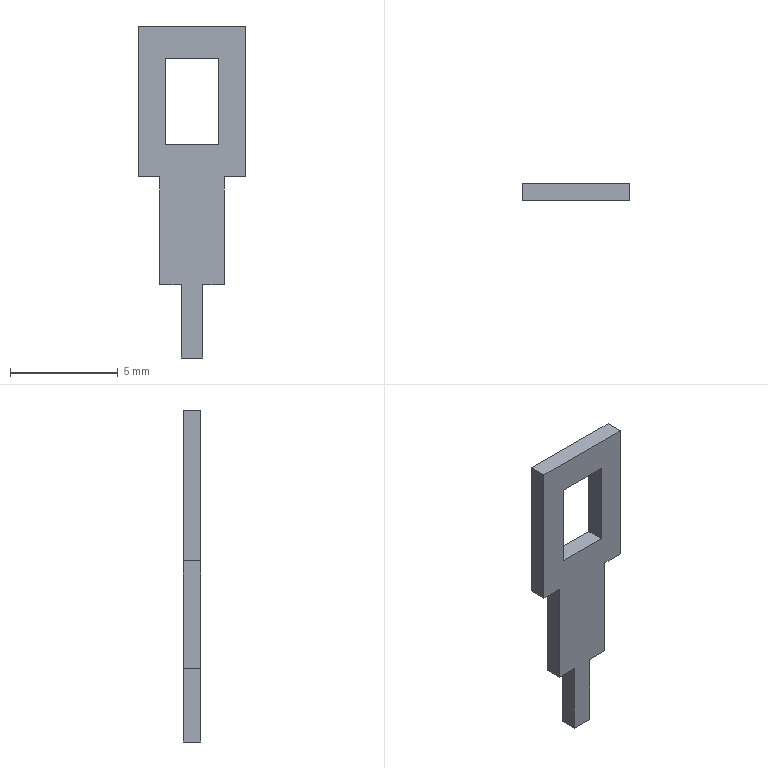Part | STEP file | LRS-150-12_X2_5F00517375-151318 | 1 solid | 18 faces | box 5 x 0.8 x 15.4 mm | volume 34.72 mm3 | plane 18
STEP:
#1=CARTESIAN_POINT('',(0.,0.,0.));
#2=DIRECTION('',(0.,0.,1.));
#3=DIRECTION('',(1.,0.,0.));
#4=AXIS2_PLACEMENT_3D('',#1,#2,#3);
#5=CARTESIAN_POINT('',(-241.667,262.225,6.5));
#6=VERTEX_POINT('',#5);
#7=CARTESIAN_POINT('',(-241.667,263.025,6.5));
#8=VERTEX_POINT('',#7);
#9=CARTESIAN_POINT('',(-241.667,262.225,6.5));
#10=DIRECTION('',(0.,1.,0.));
#11=VECTOR('',#10,1.);
#12=LINE('',#9,#11);
#13=CARTESIAN_POINT('',(-241.667,262.225,6.5));
#14=DIRECTION('',(0.,0.,1.));
#15=DIRECTION('',(1.,0.,0.));
#16=AXIS2_PLACEMENT_3D('',#13,#14,#15);
#17=PLANE('',#16);
#18=CARTESIAN_POINT('',(0.,0.));
#19=DIRECTION('',(0.,1.));
#20=VECTOR('',#19,1.);
#21=LINE('',#18,#20);
#22=(GEOMETRIC_REPRESENTATION_CONTEXT(2)PARAMETRIC_REPRESENTATION_CONTEXT()REPRESENTATION_CONTEXT('',''));
#23=DEFINITIONAL_REPRESENTATION('',(#21),#22);
#24=PCURVE('',#17,#23);
#25=CARTESIAN_POINT('',(-241.667,262.225,10.5));
#26=DIRECTION('',(-1.,0.,0.));
#27=DIRECTION('',(0.,0.,1.));
#28=AXIS2_PLACEMENT_3D('',#25,#26,#27);
#29=PLANE('',#28);
#30=CARTESIAN_POINT('',(-4.,0.));
#31=DIRECTION('',(0.,1.));
#32=VECTOR('',#31,1.);
#33=LINE('',#30,#32);
#34=(GEOMETRIC_REPRESENTATION_CONTEXT(2)PARAMETRIC_REPRESENTATION_CONTEXT()REPRESENTATION_CONTEXT('',''));
#35=DEFINITIONAL_REPRESENTATION('',(#33),#34);
#36=PCURVE('',#29,#35);
#37=SURFACE_CURVE('',#12,(#24,#36),.PCURVE_S1.);
#38=EDGE_CURVE('',#6,#8,#37,.T.);
#39=ORIENTED_EDGE('',*,*,#38,.F.);
#40=CARTESIAN_POINT('',(-244.167,262.225,6.5));
#41=VERTEX_POINT('',#40);
#42=CARTESIAN_POINT('',(-244.167,262.225,6.5));
#43=DIRECTION('',(1.,0.,0.));
#44=VECTOR('',#43,1.);
#45=LINE('',#42,#44);
#46=CARTESIAN_POINT('',(-2.5,0.));
#47=DIRECTION('',(1.,0.));
#48=VECTOR('',#47,1.);
#49=LINE('',#46,#48);
#50=(GEOMETRIC_REPRESENTATION_CONTEXT(2)PARAMETRIC_REPRESENTATION_CONTEXT()REPRESENTATION_CONTEXT('',''));
#51=DEFINITIONAL_REPRESENTATION('',(#49),#50);
#52=PCURVE('',#17,#51);
#53=CARTESIAN_POINT('',(-250.446,262.225,19.929));
#54=DIRECTION('',(0.,1.,0.));
#55=DIRECTION('',(1.,0.,0.));
#56=AXIS2_PLACEMENT_3D('',#53,#54,#55);
#57=PLANE('',#56);
#58=CARTESIAN_POINT('',(6.28,13.429));
#59=DIRECTION('',(1.,0.));
#60=VECTOR('',#59,1.);
#61=LINE('',#58,#60);
#62=(GEOMETRIC_REPRESENTATION_CONTEXT(2)PARAMETRIC_REPRESENTATION_CONTEXT()REPRESENTATION_CONTEXT('',''));
#63=DEFINITIONAL_REPRESENTATION('',(#61),#62);
#64=PCURVE('',#57,#63);
#65=SURFACE_CURVE('',#45,(#52,#64),.PCURVE_S1.);
#66=EDGE_CURVE('',#41,#6,#65,.T.);
#67=ORIENTED_EDGE('',*,*,#66,.F.);
#68=CARTESIAN_POINT('',(-244.167,263.025,6.5));
#69=VERTEX_POINT('',#68);
#70=CARTESIAN_POINT('',(-244.167,262.225,6.5));
#71=DIRECTION('',(0.,1.,0.));
#72=VECTOR('',#71,1.);
#73=LINE('',#70,#72);
#74=CARTESIAN_POINT('',(-2.5,0.));
#75=DIRECTION('',(0.,1.));
#76=VECTOR('',#75,1.);
#77=LINE('',#74,#76);
#78=(GEOMETRIC_REPRESENTATION_CONTEXT(2)PARAMETRIC_REPRESENTATION_CONTEXT()REPRESENTATION_CONTEXT('',''));
#79=DEFINITIONAL_REPRESENTATION('',(#77),#78);
#80=PCURVE('',#17,#79);
#81=CARTESIAN_POINT('',(-244.167,262.225,6.5));
#82=DIRECTION('',(1.,0.,0.));
#83=DIRECTION('',(0.,0.,-1.));
#84=AXIS2_PLACEMENT_3D('',#81,#82,#83);
#85=PLANE('',#84);
#86=CARTESIAN_POINT('',(0.,0.));
#87=DIRECTION('',(0.,1.));
#88=VECTOR('',#87,1.);
#89=LINE('',#86,#88);
#90=(GEOMETRIC_REPRESENTATION_CONTEXT(2)PARAMETRIC_REPRESENTATION_CONTEXT()REPRESENTATION_CONTEXT('',''));
#91=DEFINITIONAL_REPRESENTATION('',(#89),#90);
#92=PCURVE('',#85,#91);
#93=SURFACE_CURVE('',#73,(#80,#92),.PCURVE_S1.);
#94=EDGE_CURVE('',#41,#69,#93,.T.);
#95=ORIENTED_EDGE('',*,*,#94,.T.);
#96=CARTESIAN_POINT('',(-244.167,263.025,6.5));
#97=DIRECTION('',(1.,0.,0.));
#98=VECTOR('',#97,1.);
#99=LINE('',#96,#98);
#100=CARTESIAN_POINT('',(-2.5,0.8));
#101=DIRECTION('',(1.,0.));
#102=VECTOR('',#101,1.);
#103=LINE('',#100,#102);
#104=(GEOMETRIC_REPRESENTATION_CONTEXT(2)PARAMETRIC_REPRESENTATION_CONTEXT()REPRESENTATION_CONTEXT('',''));
#105=DEFINITIONAL_REPRESENTATION('',(#103),#104);
#106=PCURVE('',#17,#105);
#107=CARTESIAN_POINT('',(-250.446,263.025,19.929));
#108=DIRECTION('',(0.,1.,0.));
#109=DIRECTION('',(1.,0.,0.));
#110=AXIS2_PLACEMENT_3D('',#107,#108,#109);
#111=PLANE('',#110);
#112=CARTESIAN_POINT('',(6.28,13.429));
#113=DIRECTION('',(1.,0.));
#114=VECTOR('',#113,1.);
#115=LINE('',#112,#114);
#116=(GEOMETRIC_REPRESENTATION_CONTEXT(2)PARAMETRIC_REPRESENTATION_CONTEXT()REPRESENTATION_CONTEXT('',''));
#117=DEFINITIONAL_REPRESENTATION('',(#115),#116);
#118=PCURVE('',#111,#117);
#119=SURFACE_CURVE('',#99,(#106,#118),.PCURVE_S1.);
#120=EDGE_CURVE('',#69,#8,#119,.T.);
#121=ORIENTED_EDGE('',*,*,#120,.T.);
#122=EDGE_LOOP('',(#39,#67,#95,#121));
#123=FACE_BOUND('',#122,.F.);
#124=ADVANCED_FACE('',(#123),#17,.T.);
#125=CARTESIAN_POINT('',(-241.667,262.225,10.5));
#126=VERTEX_POINT('',#125);
#127=CARTESIAN_POINT('',(-241.667,263.025,10.5));
#128=VERTEX_POINT('',#127);
#129=CARTESIAN_POINT('',(-241.667,262.225,10.5));
#130=DIRECTION('',(0.,1.,0.));
#131=VECTOR('',#130,1.);
#132=LINE('',#129,#131);
#133=CARTESIAN_POINT('',(0.,0.));
#134=DIRECTION('',(0.,1.));
#135=VECTOR('',#134,1.);
#136=LINE('',#133,#135);
#137=(GEOMETRIC_REPRESENTATION_CONTEXT(2)PARAMETRIC_REPRESENTATION_CONTEXT()REPRESENTATION_CONTEXT('',''));
#138=DEFINITIONAL_REPRESENTATION('',(#136),#137);
#139=PCURVE('',#29,#138);
#140=CARTESIAN_POINT('',(-244.167,262.225,10.5));
#141=DIRECTION('',(0.,0.,-1.));
#142=DIRECTION('',(-1.,0.,0.));
#143=AXIS2_PLACEMENT_3D('',#140,#141,#142);
#144=PLANE('',#143);
#145=CARTESIAN_POINT('',(-2.5,0.));
#146=DIRECTION('',(0.,1.));
#147=VECTOR('',#146,1.);
#148=LINE('',#145,#147);
#149=(GEOMETRIC_REPRESENTATION_CONTEXT(2)PARAMETRIC_REPRESENTATION_CONTEXT()REPRESENTATION_CONTEXT('',''));
#150=DEFINITIONAL_REPRESENTATION('',(#148),#149);
#151=PCURVE('',#144,#150);
#152=SURFACE_CURVE('',#132,(#139,#151),.PCURVE_S1.);
#153=EDGE_CURVE('',#126,#128,#152,.T.);
#154=ORIENTED_EDGE('',*,*,#153,.F.);
#155=CARTESIAN_POINT('',(-241.667,262.225,6.5));
#156=DIRECTION('',(0.,0.,1.));
#157=VECTOR('',#156,1.);
#158=LINE('',#155,#157);
#159=CARTESIAN_POINT('',(-4.,0.));
#160=DIRECTION('',(1.,0.));
#161=VECTOR('',#160,1.);
#162=LINE('',#159,#161);
#163=(GEOMETRIC_REPRESENTATION_CONTEXT(2)PARAMETRIC_REPRESENTATION_CONTEXT()REPRESENTATION_CONTEXT('',''));
#164=DEFINITIONAL_REPRESENTATION('',(#162),#163);
#165=PCURVE('',#29,#164);
#166=CARTESIAN_POINT('',(8.78,13.429));
#167=DIRECTION('',(0.,-1.));
#168=VECTOR('',#167,1.);
#169=LINE('',#166,#168);
#170=(GEOMETRIC_REPRESENTATION_CONTEXT(2)PARAMETRIC_REPRESENTATION_CONTEXT()REPRESENTATION_CONTEXT('',''));
#171=DEFINITIONAL_REPRESENTATION('',(#169),#170);
#172=PCURVE('',#57,#171);
#173=SURFACE_CURVE('',#158,(#165,#172),.PCURVE_S1.);
#174=EDGE_CURVE('',#6,#126,#173,.T.);
#175=ORIENTED_EDGE('',*,*,#174,.F.);
#176=ORIENTED_EDGE('',*,*,#38,.T.);
#177=CARTESIAN_POINT('',(-241.667,263.025,6.5));
#178=DIRECTION('',(0.,0.,1.));
#179=VECTOR('',#178,1.);
#180=LINE('',#177,#179);
#181=CARTESIAN_POINT('',(-4.,0.8));
#182=DIRECTION('',(1.,0.));
#183=VECTOR('',#182,1.);
#184=LINE('',#181,#183);
#185=(GEOMETRIC_REPRESENTATION_CONTEXT(2)PARAMETRIC_REPRESENTATION_CONTEXT()REPRESENTATION_CONTEXT('',''));
#186=DEFINITIONAL_REPRESENTATION('',(#184),#185);
#187=PCURVE('',#29,#186);
#188=CARTESIAN_POINT('',(8.78,13.429));
#189=DIRECTION('',(0.,-1.));
#190=VECTOR('',#189,1.);
#191=LINE('',#188,#190);
#192=(GEOMETRIC_REPRESENTATION_CONTEXT(2)PARAMETRIC_REPRESENTATION_CONTEXT()REPRESENTATION_CONTEXT('',''));
#193=DEFINITIONAL_REPRESENTATION('',(#191),#192);
#194=PCURVE('',#111,#193);
#195=SURFACE_CURVE('',#180,(#187,#194),.PCURVE_S1.);
#196=EDGE_CURVE('',#8,#128,#195,.T.);
#197=ORIENTED_EDGE('',*,*,#196,.T.);
#198=EDGE_LOOP('',(#154,#175,#176,#197));
#199=FACE_BOUND('',#198,.F.);
#200=ADVANCED_FACE('',(#199),#29,.T.);
#201=CARTESIAN_POINT('',(-244.167,262.225,10.5));
#202=VERTEX_POINT('',#201);
#203=CARTESIAN_POINT('',(-244.167,263.025,10.5));
#204=VERTEX_POINT('',#203);
#205=CARTESIAN_POINT('',(-244.167,262.225,10.5));
#206=DIRECTION('',(0.,1.,0.));
#207=VECTOR('',#206,1.);
#208=LINE('',#205,#207);
#209=CARTESIAN_POINT('',(0.,0.));
#210=DIRECTION('',(0.,1.));
#211=VECTOR('',#210,1.);
#212=LINE('',#209,#211);
#213=(GEOMETRIC_REPRESENTATION_CONTEXT(2)PARAMETRIC_REPRESENTATION_CONTEXT()REPRESENTATION_CONTEXT('',''));
#214=DEFINITIONAL_REPRESENTATION('',(#212),#213);
#215=PCURVE('',#144,#214);
#216=CARTESIAN_POINT('',(-4.,0.));
#217=DIRECTION('',(0.,1.));
#218=VECTOR('',#217,1.);
#219=LINE('',#216,#218);
#220=(GEOMETRIC_REPRESENTATION_CONTEXT(2)PARAMETRIC_REPRESENTATION_CONTEXT()REPRESENTATION_CONTEXT('',''));
#221=DEFINITIONAL_REPRESENTATION('',(#219),#220);
#222=PCURVE('',#85,#221);
#223=SURFACE_CURVE('',#208,(#215,#222),.PCURVE_S1.);
#224=EDGE_CURVE('',#202,#204,#223,.T.);
#225=ORIENTED_EDGE('',*,*,#224,.F.);
#226=CARTESIAN_POINT('',(-241.667,262.225,10.5));
#227=DIRECTION('',(-1.,0.,0.));
#228=VECTOR('',#227,1.);
#229=LINE('',#226,#228);
#230=CARTESIAN_POINT('',(-2.5,0.));
#231=DIRECTION('',(1.,0.));
#232=VECTOR('',#231,1.);
#233=LINE('',#230,#232);
#234=(GEOMETRIC_REPRESENTATION_CONTEXT(2)PARAMETRIC_REPRESENTATION_CONTEXT()REPRESENTATION_CONTEXT('',''));
#235=DEFINITIONAL_REPRESENTATION('',(#233),#234);
#236=PCURVE('',#144,#235);
#237=CARTESIAN_POINT('',(8.78,9.429));
#238=DIRECTION('',(-1.,0.));
#239=VECTOR('',#238,1.);
#240=LINE('',#237,#239);
#241=(GEOMETRIC_REPRESENTATION_CONTEXT(2)PARAMETRIC_REPRESENTATION_CONTEXT()REPRESENTATION_CONTEXT('',''));
#242=DEFINITIONAL_REPRESENTATION('',(#240),#241);
#243=PCURVE('',#57,#242);
#244=SURFACE_CURVE('',#229,(#236,#243),.PCURVE_S1.);
#245=EDGE_CURVE('',#126,#202,#244,.T.);
#246=ORIENTED_EDGE('',*,*,#245,.F.);
#247=ORIENTED_EDGE('',*,*,#153,.T.);
#248=CARTESIAN_POINT('',(-241.667,263.025,10.5));
#249=DIRECTION('',(-1.,0.,0.));
#250=VECTOR('',#249,1.);
#251=LINE('',#248,#250);
#252=CARTESIAN_POINT('',(-2.5,0.8));
#253=DIRECTION('',(1.,0.));
#254=VECTOR('',#253,1.);
#255=LINE('',#252,#254);
#256=(GEOMETRIC_REPRESENTATION_CONTEXT(2)PARAMETRIC_REPRESENTATION_CONTEXT()REPRESENTATION_CONTEXT('',''));
#257=DEFINITIONAL_REPRESENTATION('',(#255),#256);
#258=PCURVE('',#144,#257);
#259=CARTESIAN_POINT('',(8.78,9.429));
#260=DIRECTION('',(-1.,0.));
#261=VECTOR('',#260,1.);
#262=LINE('',#259,#261);
#263=(GEOMETRIC_REPRESENTATION_CONTEXT(2)PARAMETRIC_REPRESENTATION_CONTEXT()REPRESENTATION_CONTEXT('',''));
#264=DEFINITIONAL_REPRESENTATION('',(#262),#263);
#265=PCURVE('',#111,#264);
#266=SURFACE_CURVE('',#251,(#258,#265),.PCURVE_S1.);
#267=EDGE_CURVE('',#128,#204,#266,.T.);
#268=ORIENTED_EDGE('',*,*,#267,.T.);
#269=EDGE_LOOP('',(#225,#246,#247,#268));
#270=FACE_BOUND('',#269,.F.);
#271=ADVANCED_FACE('',(#270),#144,.T.);
#272=ORIENTED_EDGE('',*,*,#94,.F.);
#273=CARTESIAN_POINT('',(-244.167,262.225,10.5));
#274=DIRECTION('',(0.,0.,-1.));
#275=VECTOR('',#274,1.);
#276=LINE('',#273,#275);
#277=CARTESIAN_POINT('',(-4.,0.));
#278=DIRECTION('',(1.,0.));
#279=VECTOR('',#278,1.);
#280=LINE('',#277,#279);
#281=(GEOMETRIC_REPRESENTATION_CONTEXT(2)PARAMETRIC_REPRESENTATION_CONTEXT()REPRESENTATION_CONTEXT('',''));
#282=DEFINITIONAL_REPRESENTATION('',(#280),#281);
#283=PCURVE('',#85,#282);
#284=CARTESIAN_POINT('',(6.28,9.429));
#285=DIRECTION('',(0.,1.));
#286=VECTOR('',#285,1.);
#287=LINE('',#284,#286);
#288=(GEOMETRIC_REPRESENTATION_CONTEXT(2)PARAMETRIC_REPRESENTATION_CONTEXT()REPRESENTATION_CONTEXT('',''));
#289=DEFINITIONAL_REPRESENTATION('',(#287),#288);
#290=PCURVE('',#57,#289);
#291=SURFACE_CURVE('',#276,(#283,#290),.PCURVE_S1.);
#292=EDGE_CURVE('',#202,#41,#291,.T.);
#293=ORIENTED_EDGE('',*,*,#292,.F.);
#294=ORIENTED_EDGE('',*,*,#224,.T.);
#295=CARTESIAN_POINT('',(-244.167,263.025,10.5));
#296=DIRECTION('',(0.,0.,-1.));
#297=VECTOR('',#296,1.);
#298=LINE('',#295,#297);
#299=CARTESIAN_POINT('',(-4.,0.8));
#300=DIRECTION('',(1.,0.));
#301=VECTOR('',#300,1.);
#302=LINE('',#299,#301);
#303=(GEOMETRIC_REPRESENTATION_CONTEXT(2)PARAMETRIC_REPRESENTATION_CONTEXT()REPRESENTATION_CONTEXT('',''));
#304=DEFINITIONAL_REPRESENTATION('',(#302),#303);
#305=PCURVE('',#85,#304);
#306=CARTESIAN_POINT('',(6.28,9.429));
#307=DIRECTION('',(0.,1.));
#308=VECTOR('',#307,1.);
#309=LINE('',#306,#308);
#310=(GEOMETRIC_REPRESENTATION_CONTEXT(2)PARAMETRIC_REPRESENTATION_CONTEXT()REPRESENTATION_CONTEXT('',''));
#311=DEFINITIONAL_REPRESENTATION('',(#309),#310);
#312=PCURVE('',#111,#311);
#313=SURFACE_CURVE('',#298,(#305,#312),.PCURVE_S1.);
#314=EDGE_CURVE('',#204,#69,#313,.T.);
#315=ORIENTED_EDGE('',*,*,#314,.T.);
#316=EDGE_LOOP('',(#272,#293,#294,#315));
#317=FACE_BOUND('',#316,.F.);
#318=ADVANCED_FACE('',(#317),#85,.T.);
#319=CARTESIAN_POINT('',(-242.417,262.225,0.));
#320=VERTEX_POINT('',#319);
#321=CARTESIAN_POINT('',(-241.417,262.225,0.));
#322=VERTEX_POINT('',#321);
#323=CARTESIAN_POINT('',(-242.417,262.225,0.));
#324=DIRECTION('',(1.,0.,0.));
#325=VECTOR('',#324,1.);
#326=LINE('',#323,#325);
#327=CARTESIAN_POINT('',(8.03,19.929));
#328=DIRECTION('',(1.,0.));
#329=VECTOR('',#328,1.);
#330=LINE('',#327,#329);
#331=(GEOMETRIC_REPRESENTATION_CONTEXT(2)PARAMETRIC_REPRESENTATION_CONTEXT()REPRESENTATION_CONTEXT('',''));
#332=DEFINITIONAL_REPRESENTATION('',(#330),#331);
#333=PCURVE('',#57,#332);
#334=CARTESIAN_POINT('',(-242.417,262.225,0.));
#335=DIRECTION('',(0.,0.,-1.));
#336=DIRECTION('',(-1.,0.,0.));
#337=AXIS2_PLACEMENT_3D('',#334,#335,#336);
#338=PLANE('',#337);
#339=CARTESIAN_POINT('',(0.,0.));
#340=DIRECTION('',(-1.,0.));
#341=VECTOR('',#340,1.);
#342=LINE('',#339,#341);
#343=(GEOMETRIC_REPRESENTATION_CONTEXT(2)PARAMETRIC_REPRESENTATION_CONTEXT()REPRESENTATION_CONTEXT('',''));
#344=DEFINITIONAL_REPRESENTATION('',(#342),#343);
#345=PCURVE('',#338,#344);
#346=SURFACE_CURVE('',#326,(#333,#345),.PCURVE_S1.);
#347=EDGE_CURVE('',#320,#322,#346,.T.);
#348=ORIENTED_EDGE('',*,*,#347,.F.);
#349=CARTESIAN_POINT('',(-242.417,262.225,-3.4));
#350=VERTEX_POINT('',#349);
#351=CARTESIAN_POINT('',(-242.417,262.225,-3.4));
#352=DIRECTION('',(0.,0.,1.));
#353=VECTOR('',#352,1.);
#354=LINE('',#351,#353);
#355=CARTESIAN_POINT('',(8.03,23.329));
#356=DIRECTION('',(0.,-1.));
#357=VECTOR('',#356,1.);
#358=LINE('',#355,#357);
#359=(GEOMETRIC_REPRESENTATION_CONTEXT(2)PARAMETRIC_REPRESENTATION_CONTEXT()REPRESENTATION_CONTEXT('',''));
#360=DEFINITIONAL_REPRESENTATION('',(#358),#359);
#361=PCURVE('',#57,#360);
#362=CARTESIAN_POINT('',(-242.417,262.225,-3.4));
#363=DIRECTION('',(1.,0.,0.));
#364=DIRECTION('',(0.,0.,-1.));
#365=AXIS2_PLACEMENT_3D('',#362,#363,#364);
#366=PLANE('',#365);
#367=CARTESIAN_POINT('',(0.,0.));
#368=DIRECTION('',(-1.,0.));
#369=VECTOR('',#368,1.);
#370=LINE('',#367,#369);
#371=(GEOMETRIC_REPRESENTATION_CONTEXT(2)PARAMETRIC_REPRESENTATION_CONTEXT()REPRESENTATION_CONTEXT('',''));
#372=DEFINITIONAL_REPRESENTATION('',(#370),#371);
#373=PCURVE('',#366,#372);
#374=SURFACE_CURVE('',#354,(#361,#373),.PCURVE_S1.);
#375=EDGE_CURVE('',#350,#320,#374,.T.);
#376=ORIENTED_EDGE('',*,*,#375,.F.);
#377=CARTESIAN_POINT('',(-243.417,262.225,-3.4));
#378=VERTEX_POINT('',#377);
#379=CARTESIAN_POINT('',(-242.417,262.225,-3.4));
#380=DIRECTION('',(-1.,0.,0.));
#381=VECTOR('',#380,1.);
#382=LINE('',#379,#381);
#383=CARTESIAN_POINT('',(8.03,23.329));
#384=DIRECTION('',(-1.,0.));
#385=VECTOR('',#384,1.);
#386=LINE('',#383,#385);
#387=(GEOMETRIC_REPRESENTATION_CONTEXT(2)PARAMETRIC_REPRESENTATION_CONTEXT()REPRESENTATION_CONTEXT('',''));
#388=DEFINITIONAL_REPRESENTATION('',(#386),#387);
#389=PCURVE('',#57,#388);
#390=CARTESIAN_POINT('',(-243.417,262.225,-3.4));
#391=DIRECTION('',(0.,0.,-1.));
#392=DIRECTION('',(-1.,0.,0.));
#393=AXIS2_PLACEMENT_3D('',#390,#391,#392);
#394=PLANE('',#393);
#395=CARTESIAN_POINT('',(-1.,0.));
#396=DIRECTION('',(1.,0.));
#397=VECTOR('',#396,1.);
#398=LINE('',#395,#397);
#399=(GEOMETRIC_REPRESENTATION_CONTEXT(2)PARAMETRIC_REPRESENTATION_CONTEXT()REPRESENTATION_CONTEXT('',''));
#400=DEFINITIONAL_REPRESENTATION('',(#398),#399);
#401=PCURVE('',#394,#400);
#402=SURFACE_CURVE('',#382,(#389,#401),.PCURVE_S1.);
#403=EDGE_CURVE('',#350,#378,#402,.T.);
#404=ORIENTED_EDGE('',*,*,#403,.T.);
#405=CARTESIAN_POINT('',(-243.417,262.225,0.));
#406=VERTEX_POINT('',#405);
#407=CARTESIAN_POINT('',(-243.417,262.225,-3.4));
#408=DIRECTION('',(0.,0.,1.));
#409=VECTOR('',#408,1.);
#410=LINE('',#407,#409);
#411=CARTESIAN_POINT('',(7.03,23.329));
#412=DIRECTION('',(0.,-1.));
#413=VECTOR('',#412,1.);
#414=LINE('',#411,#413);
#415=(GEOMETRIC_REPRESENTATION_CONTEXT(2)PARAMETRIC_REPRESENTATION_CONTEXT()REPRESENTATION_CONTEXT('',''));
#416=DEFINITIONAL_REPRESENTATION('',(#414),#415);
#417=PCURVE('',#57,#416);
#418=CARTESIAN_POINT('',(-243.417,262.225,0.));
#419=DIRECTION('',(-1.,0.,0.));
#420=DIRECTION('',(0.,0.,1.));
#421=AXIS2_PLACEMENT_3D('',#418,#419,#420);
#422=PLANE('',#421);
#423=CARTESIAN_POINT('',(-3.4,0.));
#424=DIRECTION('',(1.,0.));
#425=VECTOR('',#424,1.);
#426=LINE('',#423,#425);
#427=(GEOMETRIC_REPRESENTATION_CONTEXT(2)PARAMETRIC_REPRESENTATION_CONTEXT()REPRESENTATION_CONTEXT('',''));
#428=DEFINITIONAL_REPRESENTATION('',(#426),#427);
#429=PCURVE('',#422,#428);
#430=SURFACE_CURVE('',#410,(#417,#429),.PCURVE_S1.);
#431=EDGE_CURVE('',#378,#406,#430,.T.);
#432=ORIENTED_EDGE('',*,*,#431,.T.);
#433=CARTESIAN_POINT('',(-244.417,262.225,0.));
#434=VERTEX_POINT('',#433);
#435=CARTESIAN_POINT('',(-243.417,262.225,0.));
#436=DIRECTION('',(-1.,0.,0.));
#437=VECTOR('',#436,1.);
#438=LINE('',#435,#437);
#439=CARTESIAN_POINT('',(7.03,19.929));
#440=DIRECTION('',(-1.,0.));
#441=VECTOR('',#440,1.);
#442=LINE('',#439,#441);
#443=(GEOMETRIC_REPRESENTATION_CONTEXT(2)PARAMETRIC_REPRESENTATION_CONTEXT()REPRESENTATION_CONTEXT('',''));
#444=DEFINITIONAL_REPRESENTATION('',(#442),#443);
#445=PCURVE('',#57,#444);
#446=CARTESIAN_POINT('',(-244.417,262.225,0.));
#447=DIRECTION('',(0.,0.,-1.));
#448=DIRECTION('',(-1.,0.,0.));
#449=AXIS2_PLACEMENT_3D('',#446,#447,#448);
#450=PLANE('',#449);
#451=CARTESIAN_POINT('',(-1.,0.));
#452=DIRECTION('',(1.,0.));
#453=VECTOR('',#452,1.);
#454=LINE('',#451,#453);
#455=(GEOMETRIC_REPRESENTATION_CONTEXT(2)PARAMETRIC_REPRESENTATION_CONTEXT()REPRESENTATION_CONTEXT('',''));
#456=DEFINITIONAL_REPRESENTATION('',(#454),#455);
#457=PCURVE('',#450,#456);
#458=SURFACE_CURVE('',#438,(#445,#457),.PCURVE_S1.);
#459=EDGE_CURVE('',#406,#434,#458,.T.);
#460=ORIENTED_EDGE('',*,*,#459,.T.);
#461=CARTESIAN_POINT('',(-244.417,262.225,5.));
#462=VERTEX_POINT('',#461);
#463=CARTESIAN_POINT('',(-244.417,262.225,0.));
#464=DIRECTION('',(0.,0.,1.));
#465=VECTOR('',#464,1.);
#466=LINE('',#463,#465);
#467=CARTESIAN_POINT('',(6.03,19.929));
#468=DIRECTION('',(0.,-1.));
#469=VECTOR('',#468,1.);
#470=LINE('',#467,#469);
#471=(GEOMETRIC_REPRESENTATION_CONTEXT(2)PARAMETRIC_REPRESENTATION_CONTEXT()REPRESENTATION_CONTEXT('',''));
#472=DEFINITIONAL_REPRESENTATION('',(#470),#471);
#473=PCURVE('',#57,#472);
#474=CARTESIAN_POINT('',(-244.417,262.225,5.));
#475=DIRECTION('',(-1.,0.,0.));
#476=DIRECTION('',(0.,0.,1.));
#477=AXIS2_PLACEMENT_3D('',#474,#475,#476);
#478=PLANE('',#477);
#479=CARTESIAN_POINT('',(-5.,0.));
#480=DIRECTION('',(1.,0.));
#481=VECTOR('',#480,1.);
#482=LINE('',#479,#481);
#483=(GEOMETRIC_REPRESENTATION_CONTEXT(2)PARAMETRIC_REPRESENTATION_CONTEXT()REPRESENTATION_CONTEXT('',''));
#484=DEFINITIONAL_REPRESENTATION('',(#482),#483);
#485=PCURVE('',#478,#484);
#486=SURFACE_CURVE('',#466,(#473,#485),.PCURVE_S1.);
#487=EDGE_CURVE('',#434,#462,#486,.T.);
#488=ORIENTED_EDGE('',*,*,#487,.T.);
#489=CARTESIAN_POINT('',(-245.417,262.225,5.));
#490=VERTEX_POINT('',#489);
#491=CARTESIAN_POINT('',(-244.417,262.225,5.));
#492=DIRECTION('',(-1.,0.,0.));
#493=VECTOR('',#492,1.);
#494=LINE('',#491,#493);
#495=CARTESIAN_POINT('',(6.03,14.929));
#496=DIRECTION('',(-1.,0.));
#497=VECTOR('',#496,1.);
#498=LINE('',#495,#497);
#499=(GEOMETRIC_REPRESENTATION_CONTEXT(2)PARAMETRIC_REPRESENTATION_CONTEXT()REPRESENTATION_CONTEXT('',''));
#500=DEFINITIONAL_REPRESENTATION('',(#498),#499);
#501=PCURVE('',#57,#500);
#502=CARTESIAN_POINT('',(-245.417,262.225,5.));
#503=DIRECTION('',(0.,0.,-1.));
#504=DIRECTION('',(-1.,0.,0.));
#505=AXIS2_PLACEMENT_3D('',#502,#503,#504);
#506=PLANE('',#505);
#507=CARTESIAN_POINT('',(-1.,0.));
#508=DIRECTION('',(1.,0.));
#509=VECTOR('',#508,1.);
#510=LINE('',#507,#509);
#511=(GEOMETRIC_REPRESENTATION_CONTEXT(2)PARAMETRIC_REPRESENTATION_CONTEXT()REPRESENTATION_CONTEXT('',''));
#512=DEFINITIONAL_REPRESENTATION('',(#510),#511);
#513=PCURVE('',#506,#512);
#514=SURFACE_CURVE('',#494,(#501,#513),.PCURVE_S1.);
#515=EDGE_CURVE('',#462,#490,#514,.T.);
#516=ORIENTED_EDGE('',*,*,#515,.T.);
#517=CARTESIAN_POINT('',(-245.417,262.225,12.));
#518=VERTEX_POINT('',#517);
#519=CARTESIAN_POINT('',(-245.417,262.225,12.));
#520=DIRECTION('',(0.,0.,-1.));
#521=VECTOR('',#520,1.);
#522=LINE('',#519,#521);
#523=CARTESIAN_POINT('',(5.03,7.929));
#524=DIRECTION('',(0.,1.));
#525=VECTOR('',#524,1.);
#526=LINE('',#523,#525);
#527=(GEOMETRIC_REPRESENTATION_CONTEXT(2)PARAMETRIC_REPRESENTATION_CONTEXT()REPRESENTATION_CONTEXT('',''));
#528=DEFINITIONAL_REPRESENTATION('',(#526),#527);
#529=PCURVE('',#57,#528);
#530=CARTESIAN_POINT('',(-245.417,262.225,12.));
#531=DIRECTION('',(-1.,0.,0.));
#532=DIRECTION('',(0.,0.,1.));
#533=AXIS2_PLACEMENT_3D('',#530,#531,#532);
#534=PLANE('',#533);
#535=CARTESIAN_POINT('',(0.,0.));
#536=DIRECTION('',(-1.,0.));
#537=VECTOR('',#536,1.);
#538=LINE('',#535,#537);
#539=(GEOMETRIC_REPRESENTATION_CONTEXT(2)PARAMETRIC_REPRESENTATION_CONTEXT()REPRESENTATION_CONTEXT('',''));
#540=DEFINITIONAL_REPRESENTATION('',(#538),#539);
#541=PCURVE('',#534,#540);
#542=SURFACE_CURVE('',#522,(#529,#541),.PCURVE_S1.);
#543=EDGE_CURVE('',#518,#490,#542,.T.);
#544=ORIENTED_EDGE('',*,*,#543,.F.);
#545=CARTESIAN_POINT('',(-240.417,262.225,12.));
#546=VERTEX_POINT('',#545);
#547=CARTESIAN_POINT('',(-240.417,262.225,12.));
#548=DIRECTION('',(-1.,0.,0.));
#549=VECTOR('',#548,1.);
#550=LINE('',#547,#549);
#551=CARTESIAN_POINT('',(10.03,7.929));
#552=DIRECTION('',(-1.,0.));
#553=VECTOR('',#552,1.);
#554=LINE('',#551,#553);
#555=(GEOMETRIC_REPRESENTATION_CONTEXT(2)PARAMETRIC_REPRESENTATION_CONTEXT()REPRESENTATION_CONTEXT('',''));
#556=DEFINITIONAL_REPRESENTATION('',(#554),#555);
#557=PCURVE('',#57,#556);
#558=CARTESIAN_POINT('',(-240.417,262.225,12.));
#559=DIRECTION('',(0.,0.,1.));
#560=DIRECTION('',(1.,0.,0.));
#561=AXIS2_PLACEMENT_3D('',#558,#559,#560);
#562=PLANE('',#561);
#563=CARTESIAN_POINT('',(0.,0.));
#564=DIRECTION('',(-1.,0.));
#565=VECTOR('',#564,1.);
#566=LINE('',#563,#565);
#567=(GEOMETRIC_REPRESENTATION_CONTEXT(2)PARAMETRIC_REPRESENTATION_CONTEXT()REPRESENTATION_CONTEXT('',''));
#568=DEFINITIONAL_REPRESENTATION('',(#566),#567);
#569=PCURVE('',#562,#568);
#570=SURFACE_CURVE('',#550,(#557,#569),.PCURVE_S1.);
#571=EDGE_CURVE('',#546,#518,#570,.T.);
#572=ORIENTED_EDGE('',*,*,#571,.F.);
#573=CARTESIAN_POINT('',(-240.417,262.225,5.));
#574=VERTEX_POINT('',#573);
#575=CARTESIAN_POINT('',(-240.417,262.225,5.));
#576=DIRECTION('',(0.,0.,1.));
#577=VECTOR('',#576,1.);
#578=LINE('',#575,#577);
#579=CARTESIAN_POINT('',(10.03,14.929));
#580=DIRECTION('',(0.,-1.));
#581=VECTOR('',#580,1.);
#582=LINE('',#579,#581);
#583=(GEOMETRIC_REPRESENTATION_CONTEXT(2)PARAMETRIC_REPRESENTATION_CONTEXT()REPRESENTATION_CONTEXT('',''));
#584=DEFINITIONAL_REPRESENTATION('',(#582),#583);
#585=PCURVE('',#57,#584);
#586=CARTESIAN_POINT('',(-240.417,262.225,5.));
#587=DIRECTION('',(1.,0.,0.));
#588=DIRECTION('',(0.,0.,-1.));
#589=AXIS2_PLACEMENT_3D('',#586,#587,#588);
#590=PLANE('',#589);
#591=CARTESIAN_POINT('',(0.,0.));
#592=DIRECTION('',(-1.,0.));
#593=VECTOR('',#592,1.);
#594=LINE('',#591,#593);
#595=(GEOMETRIC_REPRESENTATION_CONTEXT(2)PARAMETRIC_REPRESENTATION_CONTEXT()REPRESENTATION_CONTEXT('',''));
#596=DEFINITIONAL_REPRESENTATION('',(#594),#595);
#597=PCURVE('',#590,#596);
#598=SURFACE_CURVE('',#578,(#585,#597),.PCURVE_S1.);
#599=EDGE_CURVE('',#574,#546,#598,.T.);
#600=ORIENTED_EDGE('',*,*,#599,.F.);
#601=CARTESIAN_POINT('',(-241.417,262.225,5.));
#602=VERTEX_POINT('',#601);
#603=CARTESIAN_POINT('',(-241.417,262.225,5.));
#604=DIRECTION('',(1.,0.,0.));
#605=VECTOR('',#604,1.);
#606=LINE('',#603,#605);
#607=CARTESIAN_POINT('',(9.03,14.929));
#608=DIRECTION('',(1.,0.));
#609=VECTOR('',#608,1.);
#610=LINE('',#607,#609);
#611=(GEOMETRIC_REPRESENTATION_CONTEXT(2)PARAMETRIC_REPRESENTATION_CONTEXT()REPRESENTATION_CONTEXT('',''));
#612=DEFINITIONAL_REPRESENTATION('',(#610),#611);
#613=PCURVE('',#57,#612);
#614=CARTESIAN_POINT('',(-241.417,262.225,5.));
#615=DIRECTION('',(0.,0.,-1.));
#616=DIRECTION('',(-1.,0.,0.));
#617=AXIS2_PLACEMENT_3D('',#614,#615,#616);
#618=PLANE('',#617);
#619=CARTESIAN_POINT('',(0.,0.));
#620=DIRECTION('',(-1.,0.));
#621=VECTOR('',#620,1.);
#622=LINE('',#619,#621);
#623=(GEOMETRIC_REPRESENTATION_CONTEXT(2)PARAMETRIC_REPRESENTATION_CONTEXT()REPRESENTATION_CONTEXT('',''));
#624=DEFINITIONAL_REPRESENTATION('',(#622),#623);
#625=PCURVE('',#618,#624);
#626=SURFACE_CURVE('',#606,(#613,#625),.PCURVE_S1.);
#627=EDGE_CURVE('',#602,#574,#626,.T.);
#628=ORIENTED_EDGE('',*,*,#627,.F.);
#629=CARTESIAN_POINT('',(-241.417,262.225,0.));
#630=DIRECTION('',(0.,0.,1.));
#631=VECTOR('',#630,1.);
#632=LINE('',#629,#631);
#633=CARTESIAN_POINT('',(9.03,19.929));
#634=DIRECTION('',(0.,-1.));
#635=VECTOR('',#634,1.);
#636=LINE('',#633,#635);
#637=(GEOMETRIC_REPRESENTATION_CONTEXT(2)PARAMETRIC_REPRESENTATION_CONTEXT()REPRESENTATION_CONTEXT('',''));
#638=DEFINITIONAL_REPRESENTATION('',(#636),#637);
#639=PCURVE('',#57,#638);
#640=CARTESIAN_POINT('',(-241.417,262.225,0.));
#641=DIRECTION('',(1.,0.,0.));
#642=DIRECTION('',(0.,0.,-1.));
#643=AXIS2_PLACEMENT_3D('',#640,#641,#642);
#644=PLANE('',#643);
#645=CARTESIAN_POINT('',(0.,0.));
#646=DIRECTION('',(-1.,0.));
#647=VECTOR('',#646,1.);
#648=LINE('',#645,#647);
#649=(GEOMETRIC_REPRESENTATION_CONTEXT(2)PARAMETRIC_REPRESENTATION_CONTEXT()REPRESENTATION_CONTEXT('',''));
#650=DEFINITIONAL_REPRESENTATION('',(#648),#649);
#651=PCURVE('',#644,#650);
#652=SURFACE_CURVE('',#632,(#639,#651),.PCURVE_S1.);
#653=EDGE_CURVE('',#322,#602,#652,.T.);
#654=ORIENTED_EDGE('',*,*,#653,.F.);
#655=EDGE_LOOP('',(#348,#376,#404,#432,#460,#488,#516,#544,#572,#600,#628,#654));
#656=FACE_BOUND('',#655,.F.);
#657=ORIENTED_EDGE('',*,*,#174,.T.);
#658=ORIENTED_EDGE('',*,*,#245,.T.);
#659=ORIENTED_EDGE('',*,*,#292,.T.);
#660=ORIENTED_EDGE('',*,*,#66,.T.);
#661=EDGE_LOOP('',(#657,#658,#659,#660));
#662=FACE_BOUND('',#661,.F.);
#663=ADVANCED_FACE('',(#656,#662),#57,.F.);
#664=CARTESIAN_POINT('',(-242.417,263.025,0.));
#665=VERTEX_POINT('',#664);
#666=CARTESIAN_POINT('',(-242.417,262.225,0.));
#667=DIRECTION('',(0.,1.,0.));
#668=VECTOR('',#667,1.);
#669=LINE('',#666,#668);
#670=CARTESIAN_POINT('',(0.,0.));
#671=DIRECTION('',(0.,1.));
#672=VECTOR('',#671,1.);
#673=LINE('',#670,#672);
#674=(GEOMETRIC_REPRESENTATION_CONTEXT(2)PARAMETRIC_REPRESENTATION_CONTEXT()REPRESENTATION_CONTEXT('',''));
#675=DEFINITIONAL_REPRESENTATION('',(#673),#674);
#676=PCURVE('',#338,#675);
#677=CARTESIAN_POINT('',(-3.4,0.));
#678=DIRECTION('',(0.,1.));
#679=VECTOR('',#678,1.);
#680=LINE('',#677,#679);
#681=(GEOMETRIC_REPRESENTATION_CONTEXT(2)PARAMETRIC_REPRESENTATION_CONTEXT()REPRESENTATION_CONTEXT('',''));
#682=DEFINITIONAL_REPRESENTATION('',(#680),#681);
#683=PCURVE('',#366,#682);
#684=SURFACE_CURVE('',#669,(#676,#683),.PCURVE_S1.);
#685=EDGE_CURVE('',#320,#665,#684,.T.);
#686=ORIENTED_EDGE('',*,*,#685,.F.);
#687=ORIENTED_EDGE('',*,*,#347,.T.);
#688=CARTESIAN_POINT('',(-241.417,263.025,0.));
#689=VERTEX_POINT('',#688);
#690=CARTESIAN_POINT('',(-241.417,262.225,0.));
#691=DIRECTION('',(0.,1.,0.));
#692=VECTOR('',#691,1.);
#693=LINE('',#690,#692);
#694=CARTESIAN_POINT('',(-1.,0.));
#695=DIRECTION('',(0.,1.));
#696=VECTOR('',#695,1.);
#697=LINE('',#694,#696);
#698=(GEOMETRIC_REPRESENTATION_CONTEXT(2)PARAMETRIC_REPRESENTATION_CONTEXT()REPRESENTATION_CONTEXT('',''));
#699=DEFINITIONAL_REPRESENTATION('',(#697),#698);
#700=PCURVE('',#338,#699);
#701=CARTESIAN_POINT('',(0.,0.));
#702=DIRECTION('',(0.,1.));
#703=VECTOR('',#702,1.);
#704=LINE('',#701,#703);
#705=(GEOMETRIC_REPRESENTATION_CONTEXT(2)PARAMETRIC_REPRESENTATION_CONTEXT()REPRESENTATION_CONTEXT('',''));
#706=DEFINITIONAL_REPRESENTATION('',(#704),#705);
#707=PCURVE('',#644,#706);
#708=SURFACE_CURVE('',#693,(#700,#707),.PCURVE_S1.);
#709=EDGE_CURVE('',#322,#689,#708,.T.);
#710=ORIENTED_EDGE('',*,*,#709,.T.);
#711=CARTESIAN_POINT('',(-242.417,263.025,0.));
#712=DIRECTION('',(1.,0.,0.));
#713=VECTOR('',#712,1.);
#714=LINE('',#711,#713);
#715=CARTESIAN_POINT('',(0.,0.8));
#716=DIRECTION('',(-1.,0.));
#717=VECTOR('',#716,1.);
#718=LINE('',#715,#717);
#719=(GEOMETRIC_REPRESENTATION_CONTEXT(2)PARAMETRIC_REPRESENTATION_CONTEXT()REPRESENTATION_CONTEXT('',''));
#720=DEFINITIONAL_REPRESENTATION('',(#718),#719);
#721=PCURVE('',#338,#720);
#722=CARTESIAN_POINT('',(8.03,19.929));
#723=DIRECTION('',(1.,0.));
#724=VECTOR('',#723,1.);
#725=LINE('',#722,#724);
#726=(GEOMETRIC_REPRESENTATION_CONTEXT(2)PARAMETRIC_REPRESENTATION_CONTEXT()REPRESENTATION_CONTEXT('',''));
#727=DEFINITIONAL_REPRESENTATION('',(#725),#726);
#728=PCURVE('',#111,#727);
#729=SURFACE_CURVE('',#714,(#721,#728),.PCURVE_S1.);
#730=EDGE_CURVE('',#665,#689,#729,.T.);
#731=ORIENTED_EDGE('',*,*,#730,.F.);
#732=EDGE_LOOP('',(#686,#687,#710,#731));
#733=FACE_BOUND('',#732,.F.);
#734=ADVANCED_FACE('',(#733),#338,.T.);
#735=CARTESIAN_POINT('',(-242.417,263.025,-3.4));
#736=VERTEX_POINT('',#735);
#737=CARTESIAN_POINT('',(-242.417,262.225,-3.4));
#738=DIRECTION('',(0.,1.,0.));
#739=VECTOR('',#738,1.);
#740=LINE('',#737,#739);
#741=CARTESIAN_POINT('',(0.,0.));
#742=DIRECTION('',(0.,1.));
#743=VECTOR('',#742,1.);
#744=LINE('',#741,#743);
#745=(GEOMETRIC_REPRESENTATION_CONTEXT(2)PARAMETRIC_REPRESENTATION_CONTEXT()REPRESENTATION_CONTEXT('',''));
#746=DEFINITIONAL_REPRESENTATION('',(#744),#745);
#747=PCURVE('',#366,#746);
#748=CARTESIAN_POINT('',(-1.,0.));
#749=DIRECTION('',(0.,1.));
#750=VECTOR('',#749,1.);
#751=LINE('',#748,#750);
#752=(GEOMETRIC_REPRESENTATION_CONTEXT(2)PARAMETRIC_REPRESENTATION_CONTEXT()REPRESENTATION_CONTEXT('',''));
#753=DEFINITIONAL_REPRESENTATION('',(#751),#752);
#754=PCURVE('',#394,#753);
#755=SURFACE_CURVE('',#740,(#747,#754),.PCURVE_S1.);
#756=EDGE_CURVE('',#350,#736,#755,.T.);
#757=ORIENTED_EDGE('',*,*,#756,.F.);
#758=ORIENTED_EDGE('',*,*,#375,.T.);
#759=ORIENTED_EDGE('',*,*,#685,.T.);
#760=CARTESIAN_POINT('',(-242.417,263.025,-3.4));
#761=DIRECTION('',(0.,0.,1.));
#762=VECTOR('',#761,1.);
#763=LINE('',#760,#762);
#764=CARTESIAN_POINT('',(0.,0.8));
#765=DIRECTION('',(-1.,0.));
#766=VECTOR('',#765,1.);
#767=LINE('',#764,#766);
#768=(GEOMETRIC_REPRESENTATION_CONTEXT(2)PARAMETRIC_REPRESENTATION_CONTEXT()REPRESENTATION_CONTEXT('',''));
#769=DEFINITIONAL_REPRESENTATION('',(#767),#768);
#770=PCURVE('',#366,#769);
#771=CARTESIAN_POINT('',(8.03,23.329));
#772=DIRECTION('',(0.,-1.));
#773=VECTOR('',#772,1.);
#774=LINE('',#771,#773);
#775=(GEOMETRIC_REPRESENTATION_CONTEXT(2)PARAMETRIC_REPRESENTATION_CONTEXT()REPRESENTATION_CONTEXT('',''));
#776=DEFINITIONAL_REPRESENTATION('',(#774),#775);
#777=PCURVE('',#111,#776);
#778=SURFACE_CURVE('',#763,(#770,#777),.PCURVE_S1.);
#779=EDGE_CURVE('',#736,#665,#778,.T.);
#780=ORIENTED_EDGE('',*,*,#779,.F.);
#781=EDGE_LOOP('',(#757,#758,#759,#780));
#782=FACE_BOUND('',#781,.F.);
#783=ADVANCED_FACE('',(#782),#366,.T.);
#784=CARTESIAN_POINT('',(-243.417,263.025,-3.4));
#785=VERTEX_POINT('',#784);
#786=CARTESIAN_POINT('',(-243.417,262.225,-3.4));
#787=DIRECTION('',(0.,1.,0.));
#788=VECTOR('',#787,1.);
#789=LINE('',#786,#788);
#790=CARTESIAN_POINT('',(0.,0.));
#791=DIRECTION('',(0.,1.));
#792=VECTOR('',#791,1.);
#793=LINE('',#790,#792);
#794=(GEOMETRIC_REPRESENTATION_CONTEXT(2)PARAMETRIC_REPRESENTATION_CONTEXT()REPRESENTATION_CONTEXT('',''));
#795=DEFINITIONAL_REPRESENTATION('',(#793),#794);
#796=PCURVE('',#394,#795);
#797=CARTESIAN_POINT('',(-3.4,0.));
#798=DIRECTION('',(0.,1.));
#799=VECTOR('',#798,1.);
#800=LINE('',#797,#799);
#801=(GEOMETRIC_REPRESENTATION_CONTEXT(2)PARAMETRIC_REPRESENTATION_CONTEXT()REPRESENTATION_CONTEXT('',''));
#802=DEFINITIONAL_REPRESENTATION('',(#800),#801);
#803=PCURVE('',#422,#802);
#804=SURFACE_CURVE('',#789,(#796,#803),.PCURVE_S1.);
#805=EDGE_CURVE('',#378,#785,#804,.T.);
#806=ORIENTED_EDGE('',*,*,#805,.F.);
#807=ORIENTED_EDGE('',*,*,#403,.F.);
#808=ORIENTED_EDGE('',*,*,#756,.T.);
#809=CARTESIAN_POINT('',(-242.417,263.025,-3.4));
#810=DIRECTION('',(-1.,0.,0.));
#811=VECTOR('',#810,1.);
#812=LINE('',#809,#811);
#813=CARTESIAN_POINT('',(-1.,0.8));
#814=DIRECTION('',(1.,0.));
#815=VECTOR('',#814,1.);
#816=LINE('',#813,#815);
#817=(GEOMETRIC_REPRESENTATION_CONTEXT(2)PARAMETRIC_REPRESENTATION_CONTEXT()REPRESENTATION_CONTEXT('',''));
#818=DEFINITIONAL_REPRESENTATION('',(#816),#817);
#819=PCURVE('',#394,#818);
#820=CARTESIAN_POINT('',(8.03,23.329));
#821=DIRECTION('',(-1.,0.));
#822=VECTOR('',#821,1.);
#823=LINE('',#820,#822);
#824=(GEOMETRIC_REPRESENTATION_CONTEXT(2)PARAMETRIC_REPRESENTATION_CONTEXT()REPRESENTATION_CONTEXT('',''));
#825=DEFINITIONAL_REPRESENTATION('',(#823),#824);
#826=PCURVE('',#111,#825);
#827=SURFACE_CURVE('',#812,(#819,#826),.PCURVE_S1.);
#828=EDGE_CURVE('',#736,#785,#827,.T.);
#829=ORIENTED_EDGE('',*,*,#828,.T.);
#830=EDGE_LOOP('',(#806,#807,#808,#829));
#831=FACE_BOUND('',#830,.F.);
#832=ADVANCED_FACE('',(#831),#394,.T.);
#833=CARTESIAN_POINT('',(-243.417,263.025,0.));
#834=VERTEX_POINT('',#833);
#835=CARTESIAN_POINT('',(-243.417,262.225,0.));
#836=DIRECTION('',(0.,1.,0.));
#837=VECTOR('',#836,1.);
#838=LINE('',#835,#837);
#839=CARTESIAN_POINT('',(0.,0.));
#840=DIRECTION('',(0.,1.));
#841=VECTOR('',#840,1.);
#842=LINE('',#839,#841);
#843=(GEOMETRIC_REPRESENTATION_CONTEXT(2)PARAMETRIC_REPRESENTATION_CONTEXT()REPRESENTATION_CONTEXT('',''));
#844=DEFINITIONAL_REPRESENTATION('',(#842),#843);
#845=PCURVE('',#422,#844);
#846=CARTESIAN_POINT('',(-1.,0.));
#847=DIRECTION('',(0.,1.));
#848=VECTOR('',#847,1.);
#849=LINE('',#846,#848);
#850=(GEOMETRIC_REPRESENTATION_CONTEXT(2)PARAMETRIC_REPRESENTATION_CONTEXT()REPRESENTATION_CONTEXT('',''));
#851=DEFINITIONAL_REPRESENTATION('',(#849),#850);
#852=PCURVE('',#450,#851);
#853=SURFACE_CURVE('',#838,(#845,#852),.PCURVE_S1.);
#854=EDGE_CURVE('',#406,#834,#853,.T.);
#855=ORIENTED_EDGE('',*,*,#854,.F.);
#856=ORIENTED_EDGE('',*,*,#431,.F.);
#857=ORIENTED_EDGE('',*,*,#805,.T.);
#858=CARTESIAN_POINT('',(-243.417,263.025,-3.4));
#859=DIRECTION('',(0.,0.,1.));
#860=VECTOR('',#859,1.);
#861=LINE('',#858,#860);
#862=CARTESIAN_POINT('',(-3.4,0.8));
#863=DIRECTION('',(1.,0.));
#864=VECTOR('',#863,1.);
#865=LINE('',#862,#864);
#866=(GEOMETRIC_REPRESENTATION_CONTEXT(2)PARAMETRIC_REPRESENTATION_CONTEXT()REPRESENTATION_CONTEXT('',''));
#867=DEFINITIONAL_REPRESENTATION('',(#865),#866);
#868=PCURVE('',#422,#867);
#869=CARTESIAN_POINT('',(7.03,23.329));
#870=DIRECTION('',(0.,-1.));
#871=VECTOR('',#870,1.);
#872=LINE('',#869,#871);
#873=(GEOMETRIC_REPRESENTATION_CONTEXT(2)PARAMETRIC_REPRESENTATION_CONTEXT()REPRESENTATION_CONTEXT('',''));
#874=DEFINITIONAL_REPRESENTATION('',(#872),#873);
#875=PCURVE('',#111,#874);
#876=SURFACE_CURVE('',#861,(#868,#875),.PCURVE_S1.);
#877=EDGE_CURVE('',#785,#834,#876,.T.);
#878=ORIENTED_EDGE('',*,*,#877,.T.);
#879=EDGE_LOOP('',(#855,#856,#857,#878));
#880=FACE_BOUND('',#879,.F.);
#881=ADVANCED_FACE('',(#880),#422,.T.);
#882=CARTESIAN_POINT('',(-244.417,263.025,0.));
#883=VERTEX_POINT('',#882);
#884=CARTESIAN_POINT('',(-244.417,262.225,0.));
#885=DIRECTION('',(0.,1.,0.));
#886=VECTOR('',#885,1.);
#887=LINE('',#884,#886);
#888=CARTESIAN_POINT('',(0.,0.));
#889=DIRECTION('',(0.,1.));
#890=VECTOR('',#889,1.);
#891=LINE('',#888,#890);
#892=(GEOMETRIC_REPRESENTATION_CONTEXT(2)PARAMETRIC_REPRESENTATION_CONTEXT()REPRESENTATION_CONTEXT('',''));
#893=DEFINITIONAL_REPRESENTATION('',(#891),#892);
#894=PCURVE('',#450,#893);
#895=CARTESIAN_POINT('',(-5.,0.));
#896=DIRECTION('',(0.,1.));
#897=VECTOR('',#896,1.);
#898=LINE('',#895,#897);
#899=(GEOMETRIC_REPRESENTATION_CONTEXT(2)PARAMETRIC_REPRESENTATION_CONTEXT()REPRESENTATION_CONTEXT('',''));
#900=DEFINITIONAL_REPRESENTATION('',(#898),#899);
#901=PCURVE('',#478,#900);
#902=SURFACE_CURVE('',#887,(#894,#901),.PCURVE_S1.);
#903=EDGE_CURVE('',#434,#883,#902,.T.);
#904=ORIENTED_EDGE('',*,*,#903,.F.);
#905=ORIENTED_EDGE('',*,*,#459,.F.);
#906=ORIENTED_EDGE('',*,*,#854,.T.);
#907=CARTESIAN_POINT('',(-243.417,263.025,0.));
#908=DIRECTION('',(-1.,0.,0.));
#909=VECTOR('',#908,1.);
#910=LINE('',#907,#909);
#911=CARTESIAN_POINT('',(-1.,0.8));
#912=DIRECTION('',(1.,0.));
#913=VECTOR('',#912,1.);
#914=LINE('',#911,#913);
#915=(GEOMETRIC_REPRESENTATION_CONTEXT(2)PARAMETRIC_REPRESENTATION_CONTEXT()REPRESENTATION_CONTEXT('',''));
#916=DEFINITIONAL_REPRESENTATION('',(#914),#915);
#917=PCURVE('',#450,#916);
#918=CARTESIAN_POINT('',(7.03,19.929));
#919=DIRECTION('',(-1.,0.));
#920=VECTOR('',#919,1.);
#921=LINE('',#918,#920);
#922=(GEOMETRIC_REPRESENTATION_CONTEXT(2)PARAMETRIC_REPRESENTATION_CONTEXT()REPRESENTATION_CONTEXT('',''));
#923=DEFINITIONAL_REPRESENTATION('',(#921),#922);
#924=PCURVE('',#111,#923);
#925=SURFACE_CURVE('',#910,(#917,#924),.PCURVE_S1.);
#926=EDGE_CURVE('',#834,#883,#925,.T.);
#927=ORIENTED_EDGE('',*,*,#926,.T.);
#928=EDGE_LOOP('',(#904,#905,#906,#927));
#929=FACE_BOUND('',#928,.F.);
#930=ADVANCED_FACE('',(#929),#450,.T.);
#931=CARTESIAN_POINT('',(-244.417,263.025,5.));
#932=VERTEX_POINT('',#931);
#933=CARTESIAN_POINT('',(-244.417,262.225,5.));
#934=DIRECTION('',(0.,1.,0.));
#935=VECTOR('',#934,1.);
#936=LINE('',#933,#935);
#937=CARTESIAN_POINT('',(0.,0.));
#938=DIRECTION('',(0.,1.));
#939=VECTOR('',#938,1.);
#940=LINE('',#937,#939);
#941=(GEOMETRIC_REPRESENTATION_CONTEXT(2)PARAMETRIC_REPRESENTATION_CONTEXT()REPRESENTATION_CONTEXT('',''));
#942=DEFINITIONAL_REPRESENTATION('',(#940),#941);
#943=PCURVE('',#478,#942);
#944=CARTESIAN_POINT('',(-1.,0.));
#945=DIRECTION('',(0.,1.));
#946=VECTOR('',#945,1.);
#947=LINE('',#944,#946);
#948=(GEOMETRIC_REPRESENTATION_CONTEXT(2)PARAMETRIC_REPRESENTATION_CONTEXT()REPRESENTATION_CONTEXT('',''));
#949=DEFINITIONAL_REPRESENTATION('',(#947),#948);
#950=PCURVE('',#506,#949);
#951=SURFACE_CURVE('',#936,(#943,#950),.PCURVE_S1.);
#952=EDGE_CURVE('',#462,#932,#951,.T.);
#953=ORIENTED_EDGE('',*,*,#952,.F.);
#954=ORIENTED_EDGE('',*,*,#487,.F.);
#955=ORIENTED_EDGE('',*,*,#903,.T.);
#956=CARTESIAN_POINT('',(-244.417,263.025,0.));
#957=DIRECTION('',(0.,0.,1.));
#958=VECTOR('',#957,1.);
#959=LINE('',#956,#958);
#960=CARTESIAN_POINT('',(-5.,0.8));
#961=DIRECTION('',(1.,0.));
#962=VECTOR('',#961,1.);
#963=LINE('',#960,#962);
#964=(GEOMETRIC_REPRESENTATION_CONTEXT(2)PARAMETRIC_REPRESENTATION_CONTEXT()REPRESENTATION_CONTEXT('',''));
#965=DEFINITIONAL_REPRESENTATION('',(#963),#964);
#966=PCURVE('',#478,#965);
#967=CARTESIAN_POINT('',(6.03,19.929));
#968=DIRECTION('',(0.,-1.));
#969=VECTOR('',#968,1.);
#970=LINE('',#967,#969);
#971=(GEOMETRIC_REPRESENTATION_CONTEXT(2)PARAMETRIC_REPRESENTATION_CONTEXT()REPRESENTATION_CONTEXT('',''));
#972=DEFINITIONAL_REPRESENTATION('',(#970),#971);
#973=PCURVE('',#111,#972);
#974=SURFACE_CURVE('',#959,(#966,#973),.PCURVE_S1.);
#975=EDGE_CURVE('',#883,#932,#974,.T.);
#976=ORIENTED_EDGE('',*,*,#975,.T.);
#977=EDGE_LOOP('',(#953,#954,#955,#976));
#978=FACE_BOUND('',#977,.F.);
#979=ADVANCED_FACE('',(#978),#478,.T.);
#980=CARTESIAN_POINT('',(-245.417,263.025,5.));
#981=VERTEX_POINT('',#980);
#982=CARTESIAN_POINT('',(-245.417,262.225,5.));
#983=DIRECTION('',(0.,1.,0.));
#984=VECTOR('',#983,1.);
#985=LINE('',#982,#984);
#986=CARTESIAN_POINT('',(0.,0.));
#987=DIRECTION('',(0.,1.));
#988=VECTOR('',#987,1.);
#989=LINE('',#986,#988);
#990=(GEOMETRIC_REPRESENTATION_CONTEXT(2)PARAMETRIC_REPRESENTATION_CONTEXT()REPRESENTATION_CONTEXT('',''));
#991=DEFINITIONAL_REPRESENTATION('',(#989),#990);
#992=PCURVE('',#506,#991);
#993=CARTESIAN_POINT('',(-7.,0.));
#994=DIRECTION('',(0.,1.));
#995=VECTOR('',#994,1.);
#996=LINE('',#993,#995);
#997=(GEOMETRIC_REPRESENTATION_CONTEXT(2)PARAMETRIC_REPRESENTATION_CONTEXT()REPRESENTATION_CONTEXT('',''));
#998=DEFINITIONAL_REPRESENTATION('',(#996),#997);
#999=PCURVE('',#534,#998);
#1000=SURFACE_CURVE('',#985,(#992,#999),.PCURVE_S1.);
#1001=EDGE_CURVE('',#490,#981,#1000,.T.);
#1002=ORIENTED_EDGE('',*,*,#1001,.F.);
#1003=ORIENTED_EDGE('',*,*,#515,.F.);
#1004=ORIENTED_EDGE('',*,*,#952,.T.);
#1005=CARTESIAN_POINT('',(-244.417,263.025,5.));
#1006=DIRECTION('',(-1.,0.,0.));
#1007=VECTOR('',#1006,1.);
#1008=LINE('',#1005,#1007);
#1009=CARTESIAN_POINT('',(-1.,0.8));
#1010=DIRECTION('',(1.,0.));
#1011=VECTOR('',#1010,1.);
#1012=LINE('',#1009,#1011);
#1013=(GEOMETRIC_REPRESENTATION_CONTEXT(2)PARAMETRIC_REPRESENTATION_CONTEXT()REPRESENTATION_CONTEXT('',''));
#1014=DEFINITIONAL_REPRESENTATION('',(#1012),#1013);
#1015=PCURVE('',#506,#1014);
#1016=CARTESIAN_POINT('',(6.03,14.929));
#1017=DIRECTION('',(-1.,0.));
#1018=VECTOR('',#1017,1.);
#1019=LINE('',#1016,#1018);
#1020=(GEOMETRIC_REPRESENTATION_CONTEXT(2)PARAMETRIC_REPRESENTATION_CONTEXT()REPRESENTATION_CONTEXT('',''));
#1021=DEFINITIONAL_REPRESENTATION('',(#1019),#1020);
#1022=PCURVE('',#111,#1021);
#1023=SURFACE_CURVE('',#1008,(#1015,#1022),.PCURVE_S1.);
#1024=EDGE_CURVE('',#932,#981,#1023,.T.);
#1025=ORIENTED_EDGE('',*,*,#1024,.T.);
#1026=EDGE_LOOP('',(#1002,#1003,#1004,#1025));
#1027=FACE_BOUND('',#1026,.F.);
#1028=ADVANCED_FACE('',(#1027),#506,.T.);
#1029=CARTESIAN_POINT('',(-245.417,263.025,12.));
#1030=VERTEX_POINT('',#1029);
#1031=CARTESIAN_POINT('',(-245.417,262.225,12.));
#1032=DIRECTION('',(0.,1.,0.));
#1033=VECTOR('',#1032,1.);
#1034=LINE('',#1031,#1033);
#1035=CARTESIAN_POINT('',(0.,0.));
#1036=DIRECTION('',(0.,1.));
#1037=VECTOR('',#1036,1.);
#1038=LINE('',#1035,#1037);
#1039=(GEOMETRIC_REPRESENTATION_CONTEXT(2)PARAMETRIC_REPRESENTATION_CONTEXT()REPRESENTATION_CONTEXT('',''));
#1040=DEFINITIONAL_REPRESENTATION('',(#1038),#1039);
#1041=PCURVE('',#534,#1040);
#1042=CARTESIAN_POINT('',(-5.,0.));
#1043=DIRECTION('',(0.,1.));
#1044=VECTOR('',#1043,1.);
#1045=LINE('',#1042,#1044);
#1046=(GEOMETRIC_REPRESENTATION_CONTEXT(2)PARAMETRIC_REPRESENTATION_CONTEXT()REPRESENTATION_CONTEXT('',''));
#1047=DEFINITIONAL_REPRESENTATION('',(#1045),#1046);
#1048=PCURVE('',#562,#1047);
#1049=SURFACE_CURVE('',#1034,(#1041,#1048),.PCURVE_S1.);
#1050=EDGE_CURVE('',#518,#1030,#1049,.T.);
#1051=ORIENTED_EDGE('',*,*,#1050,.F.);
#1052=ORIENTED_EDGE('',*,*,#543,.T.);
#1053=ORIENTED_EDGE('',*,*,#1001,.T.);
#1054=CARTESIAN_POINT('',(-245.417,263.025,12.));
#1055=DIRECTION('',(0.,0.,-1.));
#1056=VECTOR('',#1055,1.);
#1057=LINE('',#1054,#1056);
#1058=CARTESIAN_POINT('',(0.,0.8));
#1059=DIRECTION('',(-1.,0.));
#1060=VECTOR('',#1059,1.);
#1061=LINE('',#1058,#1060);
#1062=(GEOMETRIC_REPRESENTATION_CONTEXT(2)PARAMETRIC_REPRESENTATION_CONTEXT()REPRESENTATION_CONTEXT('',''));
#1063=DEFINITIONAL_REPRESENTATION('',(#1061),#1062);
#1064=PCURVE('',#534,#1063);
#1065=CARTESIAN_POINT('',(5.03,7.929));
#1066=DIRECTION('',(0.,1.));
#1067=VECTOR('',#1066,1.);
#1068=LINE('',#1065,#1067);
#1069=(GEOMETRIC_REPRESENTATION_CONTEXT(2)PARAMETRIC_REPRESENTATION_CONTEXT()REPRESENTATION_CONTEXT('',''));
#1070=DEFINITIONAL_REPRESENTATION('',(#1068),#1069);
#1071=PCURVE('',#111,#1070);
#1072=SURFACE_CURVE('',#1057,(#1064,#1071),.PCURVE_S1.);
#1073=EDGE_CURVE('',#1030,#981,#1072,.T.);
#1074=ORIENTED_EDGE('',*,*,#1073,.F.);
#1075=EDGE_LOOP('',(#1051,#1052,#1053,#1074));
#1076=FACE_BOUND('',#1075,.F.);
#1077=ADVANCED_FACE('',(#1076),#534,.T.);
#1078=CARTESIAN_POINT('',(-240.417,263.025,12.));
#1079=VERTEX_POINT('',#1078);
#1080=CARTESIAN_POINT('',(-240.417,262.225,12.));
#1081=DIRECTION('',(0.,1.,0.));
#1082=VECTOR('',#1081,1.);
#1083=LINE('',#1080,#1082);
#1084=CARTESIAN_POINT('',(0.,0.));
#1085=DIRECTION('',(0.,1.));
#1086=VECTOR('',#1085,1.);
#1087=LINE('',#1084,#1086);
#1088=(GEOMETRIC_REPRESENTATION_CONTEXT(2)PARAMETRIC_REPRESENTATION_CONTEXT()REPRESENTATION_CONTEXT('',''));
#1089=DEFINITIONAL_REPRESENTATION('',(#1087),#1088);
#1090=PCURVE('',#562,#1089);
#1091=CARTESIAN_POINT('',(-7.,0.));
#1092=DIRECTION('',(0.,1.));
#1093=VECTOR('',#1092,1.);
#1094=LINE('',#1091,#1093);
#1095=(GEOMETRIC_REPRESENTATION_CONTEXT(2)PARAMETRIC_REPRESENTATION_CONTEXT()REPRESENTATION_CONTEXT('',''));
#1096=DEFINITIONAL_REPRESENTATION('',(#1094),#1095);
#1097=PCURVE('',#590,#1096);
#1098=SURFACE_CURVE('',#1083,(#1090,#1097),.PCURVE_S1.);
#1099=EDGE_CURVE('',#546,#1079,#1098,.T.);
#1100=ORIENTED_EDGE('',*,*,#1099,.F.);
#1101=ORIENTED_EDGE('',*,*,#571,.T.);
#1102=ORIENTED_EDGE('',*,*,#1050,.T.);
#1103=CARTESIAN_POINT('',(-240.417,263.025,12.));
#1104=DIRECTION('',(-1.,0.,0.));
#1105=VECTOR('',#1104,1.);
#1106=LINE('',#1103,#1105);
#1107=CARTESIAN_POINT('',(0.,0.8));
#1108=DIRECTION('',(-1.,0.));
#1109=VECTOR('',#1108,1.);
#1110=LINE('',#1107,#1109);
#1111=(GEOMETRIC_REPRESENTATION_CONTEXT(2)PARAMETRIC_REPRESENTATION_CONTEXT()REPRESENTATION_CONTEXT('',''));
#1112=DEFINITIONAL_REPRESENTATION('',(#1110),#1111);
#1113=PCURVE('',#562,#1112);
#1114=CARTESIAN_POINT('',(10.03,7.929));
#1115=DIRECTION('',(-1.,0.));
#1116=VECTOR('',#1115,1.);
#1117=LINE('',#1114,#1116);
#1118=(GEOMETRIC_REPRESENTATION_CONTEXT(2)PARAMETRIC_REPRESENTATION_CONTEXT()REPRESENTATION_CONTEXT('',''));
#1119=DEFINITIONAL_REPRESENTATION('',(#1117),#1118);
#1120=PCURVE('',#111,#1119);
#1121=SURFACE_CURVE('',#1106,(#1113,#1120),.PCURVE_S1.);
#1122=EDGE_CURVE('',#1079,#1030,#1121,.T.);
#1123=ORIENTED_EDGE('',*,*,#1122,.F.);
#1124=EDGE_LOOP('',(#1100,#1101,#1102,#1123));
#1125=FACE_BOUND('',#1124,.F.);
#1126=ADVANCED_FACE('',(#1125),#562,.T.);
#1127=CARTESIAN_POINT('',(-240.417,263.025,5.));
#1128=VERTEX_POINT('',#1127);
#1129=CARTESIAN_POINT('',(-240.417,262.225,5.));
#1130=DIRECTION('',(0.,1.,0.));
#1131=VECTOR('',#1130,1.);
#1132=LINE('',#1129,#1131);
#1133=CARTESIAN_POINT('',(0.,0.));
#1134=DIRECTION('',(0.,1.));
#1135=VECTOR('',#1134,1.);
#1136=LINE('',#1133,#1135);
#1137=(GEOMETRIC_REPRESENTATION_CONTEXT(2)PARAMETRIC_REPRESENTATION_CONTEXT()REPRESENTATION_CONTEXT('',''));
#1138=DEFINITIONAL_REPRESENTATION('',(#1136),#1137);
#1139=PCURVE('',#590,#1138);
#1140=CARTESIAN_POINT('',(-1.,0.));
#1141=DIRECTION('',(0.,1.));
#1142=VECTOR('',#1141,1.);
#1143=LINE('',#1140,#1142);
#1144=(GEOMETRIC_REPRESENTATION_CONTEXT(2)PARAMETRIC_REPRESENTATION_CONTEXT()REPRESENTATION_CONTEXT('',''));
#1145=DEFINITIONAL_REPRESENTATION('',(#1143),#1144);
#1146=PCURVE('',#618,#1145);
#1147=SURFACE_CURVE('',#1132,(#1139,#1146),.PCURVE_S1.);
#1148=EDGE_CURVE('',#574,#1128,#1147,.T.);
#1149=ORIENTED_EDGE('',*,*,#1148,.F.);
#1150=ORIENTED_EDGE('',*,*,#599,.T.);
#1151=ORIENTED_EDGE('',*,*,#1099,.T.);
#1152=CARTESIAN_POINT('',(-240.417,263.025,5.));
#1153=DIRECTION('',(0.,0.,1.));
#1154=VECTOR('',#1153,1.);
#1155=LINE('',#1152,#1154);
#1156=CARTESIAN_POINT('',(0.,0.8));
#1157=DIRECTION('',(-1.,0.));
#1158=VECTOR('',#1157,1.);
#1159=LINE('',#1156,#1158);
#1160=(GEOMETRIC_REPRESENTATION_CONTEXT(2)PARAMETRIC_REPRESENTATION_CONTEXT()REPRESENTATION_CONTEXT('',''));
#1161=DEFINITIONAL_REPRESENTATION('',(#1159),#1160);
#1162=PCURVE('',#590,#1161);
#1163=CARTESIAN_POINT('',(10.03,14.929));
#1164=DIRECTION('',(0.,-1.));
#1165=VECTOR('',#1164,1.);
#1166=LINE('',#1163,#1165);
#1167=(GEOMETRIC_REPRESENTATION_CONTEXT(2)PARAMETRIC_REPRESENTATION_CONTEXT()REPRESENTATION_CONTEXT('',''));
#1168=DEFINITIONAL_REPRESENTATION('',(#1166),#1167);
#1169=PCURVE('',#111,#1168);
#1170=SURFACE_CURVE('',#1155,(#1162,#1169),.PCURVE_S1.);
#1171=EDGE_CURVE('',#1128,#1079,#1170,.T.);
#1172=ORIENTED_EDGE('',*,*,#1171,.F.);
#1173=EDGE_LOOP('',(#1149,#1150,#1151,#1172));
#1174=FACE_BOUND('',#1173,.F.);
#1175=ADVANCED_FACE('',(#1174),#590,.T.);
#1176=CARTESIAN_POINT('',(-241.417,263.025,5.));
#1177=VERTEX_POINT('',#1176);
#1178=CARTESIAN_POINT('',(-241.417,262.225,5.));
#1179=DIRECTION('',(0.,1.,0.));
#1180=VECTOR('',#1179,1.);
#1181=LINE('',#1178,#1180);
#1182=CARTESIAN_POINT('',(0.,0.));
#1183=DIRECTION('',(0.,1.));
#1184=VECTOR('',#1183,1.);
#1185=LINE('',#1182,#1184);
#1186=(GEOMETRIC_REPRESENTATION_CONTEXT(2)PARAMETRIC_REPRESENTATION_CONTEXT()REPRESENTATION_CONTEXT('',''));
#1187=DEFINITIONAL_REPRESENTATION('',(#1185),#1186);
#1188=PCURVE('',#618,#1187);
#1189=CARTESIAN_POINT('',(-5.,0.));
#1190=DIRECTION('',(0.,1.));
#1191=VECTOR('',#1190,1.);
#1192=LINE('',#1189,#1191);
#1193=(GEOMETRIC_REPRESENTATION_CONTEXT(2)PARAMETRIC_REPRESENTATION_CONTEXT()REPRESENTATION_CONTEXT('',''));
#1194=DEFINITIONAL_REPRESENTATION('',(#1192),#1193);
#1195=PCURVE('',#644,#1194);
#1196=SURFACE_CURVE('',#1181,(#1188,#1195),.PCURVE_S1.);
#1197=EDGE_CURVE('',#602,#1177,#1196,.T.);
#1198=ORIENTED_EDGE('',*,*,#1197,.F.);
#1199=ORIENTED_EDGE('',*,*,#627,.T.);
#1200=ORIENTED_EDGE('',*,*,#1148,.T.);
#1201=CARTESIAN_POINT('',(-241.417,263.025,5.));
#1202=DIRECTION('',(1.,0.,0.));
#1203=VECTOR('',#1202,1.);
#1204=LINE('',#1201,#1203);
#1205=CARTESIAN_POINT('',(0.,0.8));
#1206=DIRECTION('',(-1.,0.));
#1207=VECTOR('',#1206,1.);
#1208=LINE('',#1205,#1207);
#1209=(GEOMETRIC_REPRESENTATION_CONTEXT(2)PARAMETRIC_REPRESENTATION_CONTEXT()REPRESENTATION_CONTEXT('',''));
#1210=DEFINITIONAL_REPRESENTATION('',(#1208),#1209);
#1211=PCURVE('',#618,#1210);
#1212=CARTESIAN_POINT('',(9.03,14.929));
#1213=DIRECTION('',(1.,0.));
#1214=VECTOR('',#1213,1.);
#1215=LINE('',#1212,#1214);
#1216=(GEOMETRIC_REPRESENTATION_CONTEXT(2)PARAMETRIC_REPRESENTATION_CONTEXT()REPRESENTATION_CONTEXT('',''));
#1217=DEFINITIONAL_REPRESENTATION('',(#1215),#1216);
#1218=PCURVE('',#111,#1217);
#1219=SURFACE_CURVE('',#1204,(#1211,#1218),.PCURVE_S1.);
#1220=EDGE_CURVE('',#1177,#1128,#1219,.T.);
#1221=ORIENTED_EDGE('',*,*,#1220,.F.);
#1222=EDGE_LOOP('',(#1198,#1199,#1200,#1221));
#1223=FACE_BOUND('',#1222,.F.);
#1224=ADVANCED_FACE('',(#1223),#618,.T.);
#1225=ORIENTED_EDGE('',*,*,#709,.F.);
#1226=ORIENTED_EDGE('',*,*,#653,.T.);
#1227=ORIENTED_EDGE('',*,*,#1197,.T.);
#1228=CARTESIAN_POINT('',(-241.417,263.025,0.));
#1229=DIRECTION('',(0.,0.,1.));
#1230=VECTOR('',#1229,1.);
#1231=LINE('',#1228,#1230);
#1232=CARTESIAN_POINT('',(0.,0.8));
#1233=DIRECTION('',(-1.,0.));
#1234=VECTOR('',#1233,1.);
#1235=LINE('',#1232,#1234);
#1236=(GEOMETRIC_REPRESENTATION_CONTEXT(2)PARAMETRIC_REPRESENTATION_CONTEXT()REPRESENTATION_CONTEXT('',''));
#1237=DEFINITIONAL_REPRESENTATION('',(#1235),#1236);
#1238=PCURVE('',#644,#1237);
#1239=CARTESIAN_POINT('',(9.03,19.929));
#1240=DIRECTION('',(0.,-1.));
#1241=VECTOR('',#1240,1.);
#1242=LINE('',#1239,#1241);
#1243=(GEOMETRIC_REPRESENTATION_CONTEXT(2)PARAMETRIC_REPRESENTATION_CONTEXT()REPRESENTATION_CONTEXT('',''));
#1244=DEFINITIONAL_REPRESENTATION('',(#1242),#1243);
#1245=PCURVE('',#111,#1244);
#1246=SURFACE_CURVE('',#1231,(#1238,#1245),.PCURVE_S1.);
#1247=EDGE_CURVE('',#689,#1177,#1246,.T.);
#1248=ORIENTED_EDGE('',*,*,#1247,.F.);
#1249=EDGE_LOOP('',(#1225,#1226,#1227,#1248));
#1250=FACE_BOUND('',#1249,.F.);
#1251=ADVANCED_FACE('',(#1250),#644,.T.);
#1252=ORIENTED_EDGE('',*,*,#877,.F.);
#1253=ORIENTED_EDGE('',*,*,#828,.F.);
#1254=ORIENTED_EDGE('',*,*,#779,.T.);
#1255=ORIENTED_EDGE('',*,*,#730,.T.);
#1256=ORIENTED_EDGE('',*,*,#1247,.T.);
#1257=ORIENTED_EDGE('',*,*,#1220,.T.);
#1258=ORIENTED_EDGE('',*,*,#1171,.T.);
#1259=ORIENTED_EDGE('',*,*,#1122,.T.);
#1260=ORIENTED_EDGE('',*,*,#1073,.T.);
#1261=ORIENTED_EDGE('',*,*,#1024,.F.);
#1262=ORIENTED_EDGE('',*,*,#975,.F.);
#1263=ORIENTED_EDGE('',*,*,#926,.F.);
#1264=EDGE_LOOP('',(#1252,#1253,#1254,#1255,#1256,#1257,#1258,#1259,#1260,#1261,#1262,#1263));
#1265=FACE_BOUND('',#1264,.F.);
#1266=ORIENTED_EDGE('',*,*,#120,.F.);
#1267=ORIENTED_EDGE('',*,*,#314,.F.);
#1268=ORIENTED_EDGE('',*,*,#267,.F.);
#1269=ORIENTED_EDGE('',*,*,#196,.F.);
#1270=EDGE_LOOP('',(#1266,#1267,#1268,#1269));
#1271=FACE_BOUND('',#1270,.F.);
#1272=ADVANCED_FACE('',(#1265,#1271),#111,.T.);
#1273=CLOSED_SHELL('',(#124,#200,#271,#318,#663,#734,#783,#832,#881,#930,#979,#1028,#1077,#1126,#1175,#1224,#1251,#1272));
#1274=MANIFOLD_SOLID_BREP('',#1273);
#1275=(LENGTH_UNIT()NAMED_UNIT(*)SI_UNIT(.MILLI.,.METRE.));
#1276=UNCERTAINTY_MEASURE_WITH_UNIT(LENGTH_MEASURE(0.0000001),#1275,'','');
#1277=(NAMED_UNIT(*)PLANE_ANGLE_UNIT()SI_UNIT($,.RADIAN.));
#1278=(NAMED_UNIT(*)SI_UNIT($,.STERADIAN.)SOLID_ANGLE_UNIT());
#1279=(GEOMETRIC_REPRESENTATION_CONTEXT(3)GLOBAL_UNCERTAINTY_ASSIGNED_CONTEXT((#1276))GLOBAL_UNIT_ASSIGNED_CONTEXT((#1275,#1277,#1278))REPRESENTATION_CONTEXT('',''));
#1280=ADVANCED_BREP_SHAPE_REPRESENTATION('',(#4,#1274),#1279);